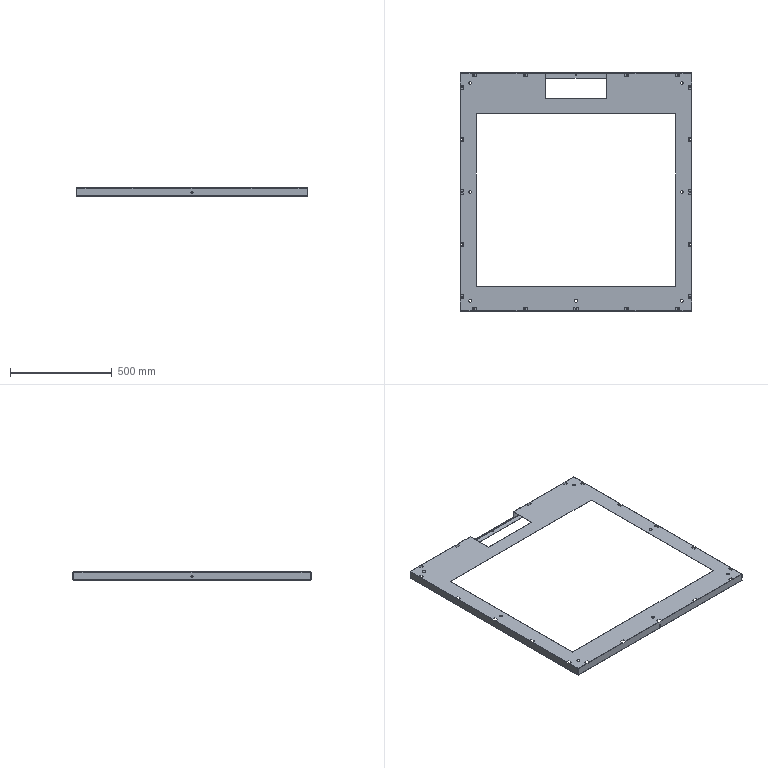Part | 1 solid | 384 faces | box 1139 x 1169 x 40 mm | volume 738169 mm3 | plane 242 | cylinder 126 | spline 16 | commonest cylinder face diameters 7 x50 0.4 x28 2.4 x28 14 x14 10 x6